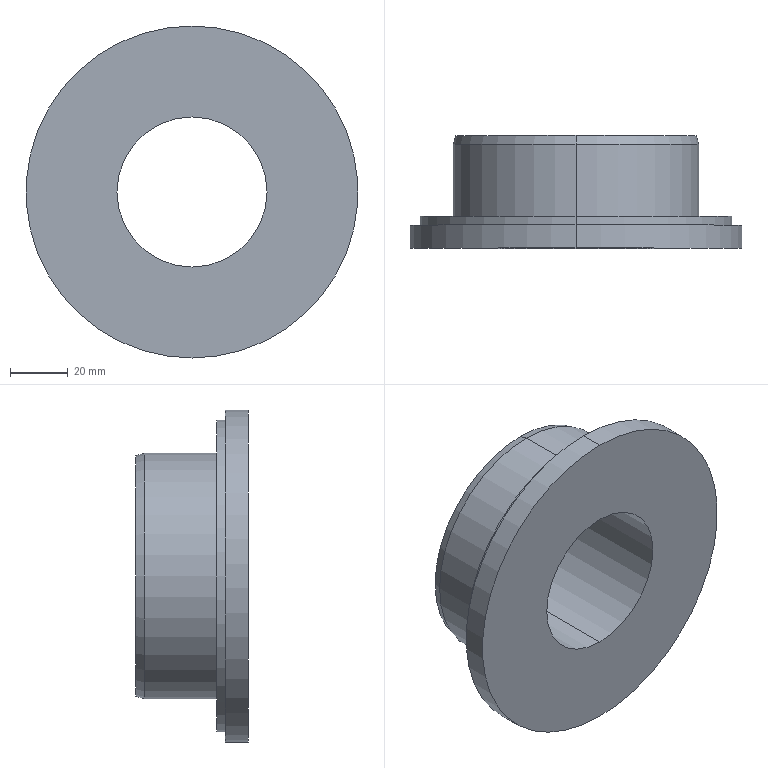Part | SolidWorks | features Chamfer 1, Revolution 1 | 1 solid | 14 faces | box 115 x 39 x 115 mm | volume 186319 mm3 | cylinder 8 | plane 4 | cone 2 | commonest cylinder face diameters 52 x2 85 x2 108 x2 115 x2
STEP:
#1=CARTESIAN_POINT('',(0.,31.,41.696));
#2=VERTEX_POINT('',#1);
#3=CARTESIAN_POINT('',(0.,31.,-41.696));
#4=VERTEX_POINT('',#3);
#5=CARTESIAN_POINT('',(0.,31.,0.));
#6=DIRECTION('',(0.,1.,0.));
#7=DIRECTION('',(0.,0.,1.));
#8=AXIS2_PLACEMENT_3D('',#5,#6,#7);
#9=CIRCLE('',#8,41.696);
#10=EDGE_CURVE('',#2,#4,#9,.T.);
#11=ORIENTED_EDGE('',*,*,#10,.F.);
#12=CARTESIAN_POINT('',(0.,28.,42.5));
#13=VERTEX_POINT('',#12);
#14=CARTESIAN_POINT('',(0.,28.,42.5));
#15=DIRECTION('',(0.,-0.9659,0.2588));
#16=VECTOR('',#15,1000.);
#17=LINE('',#14,#16);
#18=EDGE_CURVE('',#2,#13,#17,.T.);
#19=ORIENTED_EDGE('',*,*,#18,.T.);
#20=CARTESIAN_POINT('',(0.,28.,-42.5));
#21=VERTEX_POINT('',#20);
#22=CARTESIAN_POINT('',(0.,28.,0.));
#23=DIRECTION('',(0.,-1.,0.));
#24=DIRECTION('',(0.,0.,1.));
#25=AXIS2_PLACEMENT_3D('',#22,#23,#24);
#26=CIRCLE('',#25,42.5);
#27=EDGE_CURVE('',#21,#13,#26,.T.);
#28=ORIENTED_EDGE('',*,*,#27,.F.);
#29=CARTESIAN_POINT('',(0.,28.,-42.5));
#30=DIRECTION('',(0.,-0.9659,-0.2588));
#31=VECTOR('',#30,1000.);
#32=LINE('',#29,#31);
#33=EDGE_CURVE('',#4,#21,#32,.T.);
#34=ORIENTED_EDGE('',*,*,#33,.F.);
#35=EDGE_LOOP('',(#11,#19,#28,#34));
#36=FACE_OUTER_BOUND('',#35,.T.);
#37=CARTESIAN_POINT('',(0.,28.,0.));
#38=DIRECTION('',(0.,-1.,0.));
#39=DIRECTION('',(0.,0.,-1.));
#40=AXIS2_PLACEMENT_3D('',#37,#38,#39);
#41=CONICAL_SURFACE('',#40,42.5,0.2618);
#42=ADVANCED_FACE('',(#36),#41,.T.);
#43=CARTESIAN_POINT('',(0.,3.,-54.));
#44=VERTEX_POINT('',#43);
#45=CARTESIAN_POINT('',(0.,3.,54.));
#46=VERTEX_POINT('',#45);
#47=CARTESIAN_POINT('',(0.,3.,0.));
#48=DIRECTION('',(0.,-1.,0.));
#49=DIRECTION('',(0.,0.,-1.));
#50=AXIS2_PLACEMENT_3D('',#47,#48,#49);
#51=CIRCLE('',#50,54.);
#52=EDGE_CURVE('',#44,#46,#51,.T.);
#53=ORIENTED_EDGE('',*,*,#52,.T.);
#54=CARTESIAN_POINT('',(0.,0.,54.));
#55=VERTEX_POINT('',#54);
#56=CARTESIAN_POINT('',(0.,0.,54.));
#57=DIRECTION('',(0.,-1.,0.));
#58=VECTOR('',#57,1000.);
#59=LINE('',#56,#58);
#60=EDGE_CURVE('',#46,#55,#59,.T.);
#61=ORIENTED_EDGE('',*,*,#60,.T.);
#62=CARTESIAN_POINT('',(0.,0.,-54.));
#63=VERTEX_POINT('',#62);
#64=CARTESIAN_POINT('',(0.,0.,0.));
#65=DIRECTION('',(0.,-1.,0.));
#66=DIRECTION('',(0.,0.,-1.));
#67=AXIS2_PLACEMENT_3D('',#64,#65,#66);
#68=CIRCLE('',#67,54.);
#69=EDGE_CURVE('',#63,#55,#68,.T.);
#70=ORIENTED_EDGE('',*,*,#69,.F.);
#71=CARTESIAN_POINT('',(0.,0.,-54.));
#72=DIRECTION('',(0.,-1.,0.));
#73=VECTOR('',#72,1000.);
#74=LINE('',#71,#73);
#75=EDGE_CURVE('',#44,#63,#74,.T.);
#76=ORIENTED_EDGE('',*,*,#75,.F.);
#77=EDGE_LOOP('',(#53,#61,#70,#76));
#78=FACE_OUTER_BOUND('',#77,.T.);
#79=CARTESIAN_POINT('',(0.,0.,0.));
#80=DIRECTION('',(0.,-1.,0.));
#81=DIRECTION('',(0.,0.,-1.));
#82=AXIS2_PLACEMENT_3D('',#79,#80,#81);
#83=CYLINDRICAL_SURFACE('',#82,54.);
#84=ADVANCED_FACE('',(#78),#83,.T.);
#85=CARTESIAN_POINT('',(0.,0.,-57.5));
#86=VERTEX_POINT('',#85);
#87=CARTESIAN_POINT('',(0.,0.,57.5));
#88=VERTEX_POINT('',#87);
#89=CARTESIAN_POINT('',(0.,0.,0.));
#90=DIRECTION('',(0.,-1.,0.));
#91=DIRECTION('',(0.,0.,-1.));
#92=AXIS2_PLACEMENT_3D('',#89,#90,#91);
#93=CIRCLE('',#92,57.5);
#94=EDGE_CURVE('',#86,#88,#93,.T.);
#95=ORIENTED_EDGE('',*,*,#94,.T.);
#96=CARTESIAN_POINT('',(0.,-8.,57.5));
#97=VERTEX_POINT('',#96);
#98=CARTESIAN_POINT('',(0.,0.,57.5));
#99=DIRECTION('',(0.,-1.,0.));
#100=VECTOR('',#99,1000.);
#101=LINE('',#98,#100);
#102=EDGE_CURVE('',#88,#97,#101,.T.);
#103=ORIENTED_EDGE('',*,*,#102,.T.);
#104=CARTESIAN_POINT('',(0.,-8.,-57.5));
#105=VERTEX_POINT('',#104);
#106=CARTESIAN_POINT('',(0.,-8.,0.));
#107=DIRECTION('',(0.,-1.,0.));
#108=DIRECTION('',(0.,0.,-1.));
#109=AXIS2_PLACEMENT_3D('',#106,#107,#108);
#110=CIRCLE('',#109,57.5);
#111=EDGE_CURVE('',#105,#97,#110,.T.);
#112=ORIENTED_EDGE('',*,*,#111,.F.);
#113=CARTESIAN_POINT('',(0.,0.,-57.5));
#114=DIRECTION('',(0.,-1.,0.));
#115=VECTOR('',#114,1000.);
#116=LINE('',#113,#115);
#117=EDGE_CURVE('',#86,#105,#116,.T.);
#118=ORIENTED_EDGE('',*,*,#117,.F.);
#119=EDGE_LOOP('',(#95,#103,#112,#118));
#120=FACE_OUTER_BOUND('',#119,.T.);
#121=CARTESIAN_POINT('',(0.,0.,0.));
#122=DIRECTION('',(0.,-1.,0.));
#123=DIRECTION('',(0.,0.,-1.));
#124=AXIS2_PLACEMENT_3D('',#121,#122,#123);
#125=CYLINDRICAL_SURFACE('',#124,57.5);
#126=ADVANCED_FACE('',(#120),#125,.T.);
#127=CARTESIAN_POINT('',(0.,31.,26.));
#128=VERTEX_POINT('',#127);
#129=CARTESIAN_POINT('',(0.,31.,-26.));
#130=VERTEX_POINT('',#129);
#131=CARTESIAN_POINT('',(0.,31.,0.));
#132=DIRECTION('',(0.,-1.,0.));
#133=DIRECTION('',(0.,0.,-1.));
#134=AXIS2_PLACEMENT_3D('',#131,#132,#133);
#135=CIRCLE('',#134,26.);
#136=EDGE_CURVE('',#128,#130,#135,.T.);
#137=ORIENTED_EDGE('',*,*,#136,.F.);
#138=CARTESIAN_POINT('',(0.,-8.,26.));
#139=VERTEX_POINT('',#138);
#140=CARTESIAN_POINT('',(0.,0.,26.));
#141=DIRECTION('',(0.,-1.,0.));
#142=VECTOR('',#141,1000.);
#143=LINE('',#140,#142);
#144=EDGE_CURVE('',#128,#139,#143,.T.);
#145=ORIENTED_EDGE('',*,*,#144,.T.);
#146=CARTESIAN_POINT('',(0.,-8.,-26.));
#147=VERTEX_POINT('',#146);
#148=CARTESIAN_POINT('',(0.,-8.,0.));
#149=DIRECTION('',(0.,-1.,0.));
#150=DIRECTION('',(0.,0.,-1.));
#151=AXIS2_PLACEMENT_3D('',#148,#149,#150);
#152=CIRCLE('',#151,26.);
#153=EDGE_CURVE('',#139,#147,#152,.T.);
#154=ORIENTED_EDGE('',*,*,#153,.T.);
#155=CARTESIAN_POINT('',(0.,0.,-26.));
#156=DIRECTION('',(0.,-1.,0.));
#157=VECTOR('',#156,1000.);
#158=LINE('',#155,#157);
#159=EDGE_CURVE('',#130,#147,#158,.T.);
#160=ORIENTED_EDGE('',*,*,#159,.F.);
#161=EDGE_LOOP('',(#137,#145,#154,#160));
#162=FACE_OUTER_BOUND('',#161,.T.);
#163=CARTESIAN_POINT('',(0.,0.,0.));
#164=DIRECTION('',(0.,-1.,0.));
#165=DIRECTION('',(0.,0.,-1.));
#166=AXIS2_PLACEMENT_3D('',#163,#164,#165);
#167=CYLINDRICAL_SURFACE('',#166,26.);
#168=ADVANCED_FACE('',(#162),#167,.F.);
#169=ORIENTED_EDGE('',*,*,#27,.T.);
#170=CARTESIAN_POINT('',(0.,3.,42.5));
#171=VERTEX_POINT('',#170);
#172=CARTESIAN_POINT('',(0.,0.,42.5));
#173=DIRECTION('',(0.,-1.,0.));
#174=VECTOR('',#173,1000.);
#175=LINE('',#172,#174);
#176=EDGE_CURVE('',#13,#171,#175,.T.);
#177=ORIENTED_EDGE('',*,*,#176,.T.);
#178=CARTESIAN_POINT('',(0.,3.,-42.5));
#179=VERTEX_POINT('',#178);
#180=CARTESIAN_POINT('',(0.,3.,0.));
#181=DIRECTION('',(0.,-1.,0.));
#182=DIRECTION('',(0.,0.,-1.));
#183=AXIS2_PLACEMENT_3D('',#180,#181,#182);
#184=CIRCLE('',#183,42.5);
#185=EDGE_CURVE('',#179,#171,#184,.T.);
#186=ORIENTED_EDGE('',*,*,#185,.F.);
#187=CARTESIAN_POINT('',(0.,0.,-42.5));
#188=DIRECTION('',(0.,-1.,0.));
#189=VECTOR('',#188,1000.);
#190=LINE('',#187,#189);
#191=EDGE_CURVE('',#21,#179,#190,.T.);
#192=ORIENTED_EDGE('',*,*,#191,.F.);
#193=EDGE_LOOP('',(#169,#177,#186,#192));
#194=FACE_OUTER_BOUND('',#193,.T.);
#195=CARTESIAN_POINT('',(0.,0.,0.));
#196=DIRECTION('',(0.,-1.,0.));
#197=DIRECTION('',(0.,0.,-1.));
#198=AXIS2_PLACEMENT_3D('',#195,#196,#197);
#199=CYLINDRICAL_SURFACE('',#198,42.5);
#200=ADVANCED_FACE('',(#194),#199,.T.);
#201=ORIENTED_EDGE('',*,*,#176,.F.);
#202=CARTESIAN_POINT('',(0.,28.,0.));
#203=DIRECTION('',(0.,-1.,0.));
#204=DIRECTION('',(0.,0.,1.));
#205=AXIS2_PLACEMENT_3D('',#202,#203,#204);
#206=CIRCLE('',#205,42.5);
#207=EDGE_CURVE('',#13,#21,#206,.T.);
#208=ORIENTED_EDGE('',*,*,#207,.T.);
#209=ORIENTED_EDGE('',*,*,#191,.T.);
#210=CARTESIAN_POINT('',(0.,3.,0.));
#211=DIRECTION('',(0.,-1.,0.));
#212=DIRECTION('',(0.,0.,-1.));
#213=AXIS2_PLACEMENT_3D('',#210,#211,#212);
#214=CIRCLE('',#213,42.5);
#215=EDGE_CURVE('',#171,#179,#214,.T.);
#216=ORIENTED_EDGE('',*,*,#215,.F.);
#217=EDGE_LOOP('',(#201,#208,#209,#216));
#218=FACE_OUTER_BOUND('',#217,.T.);
#219=CARTESIAN_POINT('',(0.,0.,0.));
#220=DIRECTION('',(0.,-1.,0.));
#221=DIRECTION('',(0.,0.,-1.));
#222=AXIS2_PLACEMENT_3D('',#219,#220,#221);
#223=CYLINDRICAL_SURFACE('',#222,42.5);
#224=ADVANCED_FACE('',(#218),#223,.T.);
#225=CARTESIAN_POINT('',(0.,31.,0.));
#226=DIRECTION('',(0.,1.,0.));
#227=DIRECTION('',(0.,0.,1.));
#228=AXIS2_PLACEMENT_3D('',#225,#226,#227);
#229=CIRCLE('',#228,41.696);
#230=EDGE_CURVE('',#4,#2,#229,.T.);
#231=ORIENTED_EDGE('',*,*,#230,.T.);
#232=ORIENTED_EDGE('',*,*,#10,.T.);
#233=EDGE_LOOP('',(#231,#232));
#234=FACE_OUTER_BOUND('',#233,.T.);
#235=CARTESIAN_POINT('',(0.,31.,0.));
#236=DIRECTION('',(0.,-1.,0.));
#237=DIRECTION('',(0.,0.,-1.));
#238=AXIS2_PLACEMENT_3D('',#235,#236,#237);
#239=CIRCLE('',#238,26.);
#240=EDGE_CURVE('',#130,#128,#239,.T.);
#241=ORIENTED_EDGE('',*,*,#240,.T.);
#242=ORIENTED_EDGE('',*,*,#136,.T.);
#243=EDGE_LOOP('',(#241,#242));
#244=FACE_BOUND('',#243,.T.);
#245=CARTESIAN_POINT('',(26.,31.,0.));
#246=DIRECTION('',(0.,1.,0.));
#247=DIRECTION('',(0.,0.,1.));
#248=AXIS2_PLACEMENT_3D('',#245,#246,#247);
#249=PLANE('',#248);
#250=ADVANCED_FACE('',(#234,#244),#249,.T.);
#251=ORIENTED_EDGE('',*,*,#144,.F.);
#252=ORIENTED_EDGE('',*,*,#240,.F.);
#253=ORIENTED_EDGE('',*,*,#159,.T.);
#254=CARTESIAN_POINT('',(0.,-8.,0.));
#255=DIRECTION('',(0.,-1.,0.));
#256=DIRECTION('',(0.,0.,-1.));
#257=AXIS2_PLACEMENT_3D('',#254,#255,#256);
#258=CIRCLE('',#257,26.);
#259=EDGE_CURVE('',#147,#139,#258,.T.);
#260=ORIENTED_EDGE('',*,*,#259,.T.);
#261=EDGE_LOOP('',(#251,#252,#253,#260));
#262=FACE_OUTER_BOUND('',#261,.T.);
#263=CARTESIAN_POINT('',(0.,0.,0.));
#264=DIRECTION('',(0.,-1.,0.));
#265=DIRECTION('',(0.,0.,-1.));
#266=AXIS2_PLACEMENT_3D('',#263,#264,#265);
#267=CYLINDRICAL_SURFACE('',#266,26.);
#268=ADVANCED_FACE('',(#262),#267,.F.);
#269=ORIENTED_EDGE('',*,*,#111,.T.);
#270=CARTESIAN_POINT('',(0.,-8.,0.));
#271=DIRECTION('',(0.,-1.,0.));
#272=DIRECTION('',(0.,0.,-1.));
#273=AXIS2_PLACEMENT_3D('',#270,#271,#272);
#274=CIRCLE('',#273,57.5);
#275=EDGE_CURVE('',#97,#105,#274,.T.);
#276=ORIENTED_EDGE('',*,*,#275,.T.);
#277=EDGE_LOOP('',(#269,#276));
#278=FACE_OUTER_BOUND('',#277,.T.);
#279=ORIENTED_EDGE('',*,*,#259,.F.);
#280=ORIENTED_EDGE('',*,*,#153,.F.);
#281=EDGE_LOOP('',(#279,#280));
#282=FACE_BOUND('',#281,.T.);
#283=CARTESIAN_POINT('',(57.5,-8.,0.));
#284=DIRECTION('',(0.,-1.,0.));
#285=DIRECTION('',(0.,0.,-1.));
#286=AXIS2_PLACEMENT_3D('',#283,#284,#285);
#287=PLANE('',#286);
#288=ADVANCED_FACE('',(#278,#282),#287,.T.);
#289=ORIENTED_EDGE('',*,*,#102,.F.);
#290=CARTESIAN_POINT('',(0.,0.,0.));
#291=DIRECTION('',(0.,-1.,0.));
#292=DIRECTION('',(0.,0.,-1.));
#293=AXIS2_PLACEMENT_3D('',#290,#291,#292);
#294=CIRCLE('',#293,57.5);
#295=EDGE_CURVE('',#88,#86,#294,.T.);
#296=ORIENTED_EDGE('',*,*,#295,.T.);
#297=ORIENTED_EDGE('',*,*,#117,.T.);
#298=ORIENTED_EDGE('',*,*,#275,.F.);
#299=EDGE_LOOP('',(#289,#296,#297,#298));
#300=FACE_OUTER_BOUND('',#299,.T.);
#301=CARTESIAN_POINT('',(0.,0.,0.));
#302=DIRECTION('',(0.,-1.,0.));
#303=DIRECTION('',(0.,0.,-1.));
#304=AXIS2_PLACEMENT_3D('',#301,#302,#303);
#305=CYLINDRICAL_SURFACE('',#304,57.5);
#306=ADVANCED_FACE('',(#300),#305,.T.);
#307=ORIENTED_EDGE('',*,*,#69,.T.);
#308=CARTESIAN_POINT('',(0.,0.,0.));
#309=DIRECTION('',(0.,-1.,0.));
#310=DIRECTION('',(0.,0.,-1.));
#311=AXIS2_PLACEMENT_3D('',#308,#309,#310);
#312=CIRCLE('',#311,54.);
#313=EDGE_CURVE('',#55,#63,#312,.T.);
#314=ORIENTED_EDGE('',*,*,#313,.T.);
#315=EDGE_LOOP('',(#307,#314));
#316=FACE_BOUND('',#315,.T.);
#317=ORIENTED_EDGE('',*,*,#94,.F.);
#318=ORIENTED_EDGE('',*,*,#295,.F.);
#319=EDGE_LOOP('',(#317,#318));
#320=FACE_OUTER_BOUND('',#319,.T.);
#321=CARTESIAN_POINT('',(54.,0.,0.));
#322=DIRECTION('',(0.,1.,0.));
#323=DIRECTION('',(0.,0.,1.));
#324=AXIS2_PLACEMENT_3D('',#321,#322,#323);
#325=PLANE('',#324);
#326=ADVANCED_FACE('',(#316,#320),#325,.T.);
#327=ORIENTED_EDGE('',*,*,#60,.F.);
#328=CARTESIAN_POINT('',(0.,3.,0.));
#329=DIRECTION('',(0.,-1.,0.));
#330=DIRECTION('',(0.,0.,-1.));
#331=AXIS2_PLACEMENT_3D('',#328,#329,#330);
#332=CIRCLE('',#331,54.);
#333=EDGE_CURVE('',#46,#44,#332,.T.);
#334=ORIENTED_EDGE('',*,*,#333,.T.);
#335=ORIENTED_EDGE('',*,*,#75,.T.);
#336=ORIENTED_EDGE('',*,*,#313,.F.);
#337=EDGE_LOOP('',(#327,#334,#335,#336));
#338=FACE_OUTER_BOUND('',#337,.T.);
#339=CARTESIAN_POINT('',(0.,0.,0.));
#340=DIRECTION('',(0.,-1.,0.));
#341=DIRECTION('',(0.,0.,-1.));
#342=AXIS2_PLACEMENT_3D('',#339,#340,#341);
#343=CYLINDRICAL_SURFACE('',#342,54.);
#344=ADVANCED_FACE('',(#338),#343,.T.);
#345=ORIENTED_EDGE('',*,*,#185,.T.);
#346=ORIENTED_EDGE('',*,*,#215,.T.);
#347=EDGE_LOOP('',(#345,#346));
#348=FACE_BOUND('',#347,.T.);
#349=ORIENTED_EDGE('',*,*,#52,.F.);
#350=ORIENTED_EDGE('',*,*,#333,.F.);
#351=EDGE_LOOP('',(#349,#350));
#352=FACE_OUTER_BOUND('',#351,.T.);
#353=CARTESIAN_POINT('',(42.5,3.,0.));
#354=DIRECTION('',(0.,1.,0.));
#355=DIRECTION('',(0.,0.,1.));
#356=AXIS2_PLACEMENT_3D('',#353,#354,#355);
#357=PLANE('',#356);
#358=ADVANCED_FACE('',(#348,#352),#357,.T.);
#359=ORIENTED_EDGE('',*,*,#18,.F.);
#360=ORIENTED_EDGE('',*,*,#230,.F.);
#361=ORIENTED_EDGE('',*,*,#33,.T.);
#362=ORIENTED_EDGE('',*,*,#207,.F.);
#363=EDGE_LOOP('',(#359,#360,#361,#362));
#364=FACE_OUTER_BOUND('',#363,.T.);
#365=CARTESIAN_POINT('',(0.,28.,0.));
#366=DIRECTION('',(0.,-1.,0.));
#367=DIRECTION('',(0.,0.,-1.));
#368=AXIS2_PLACEMENT_3D('',#365,#366,#367);
#369=CONICAL_SURFACE('',#368,42.5,0.2618);
#370=ADVANCED_FACE('',(#364),#369,.T.);
#371=CLOSED_SHELL('',(#42,#84,#126,#168,#200,#224,#250,#268,#288,#306,#326,#344,#358,#370));
#372=MANIFOLD_SOLID_BREP('',#371);
#373=CARTESIAN_POINT('',(0.,0.,0.));
#374=DIRECTION('',(0.,0.,1.));
#375=DIRECTION('',(1.,0.,0.));
#376=AXIS2_PLACEMENT_3D('',#373,#374,#375);
#377=(LENGTH_UNIT()NAMED_UNIT(*)SI_UNIT(.MILLI.,.METRE.));
#378=UNCERTAINTY_MEASURE_WITH_UNIT(LENGTH_MEASURE(0.00001),#377,'','');
#379=(NAMED_UNIT(*)PLANE_ANGLE_UNIT()SI_UNIT($,.RADIAN.));
#380=(NAMED_UNIT(*)SI_UNIT($,.STERADIAN.)SOLID_ANGLE_UNIT());
#381=(GEOMETRIC_REPRESENTATION_CONTEXT(3)GLOBAL_UNCERTAINTY_ASSIGNED_CONTEXT((#378))GLOBAL_UNIT_ASSIGNED_CONTEXT((#377,#379,#380))REPRESENTATION_CONTEXT('',''));
#382=ADVANCED_BREP_SHAPE_REPRESENTATION('',(#372,#376),#381);